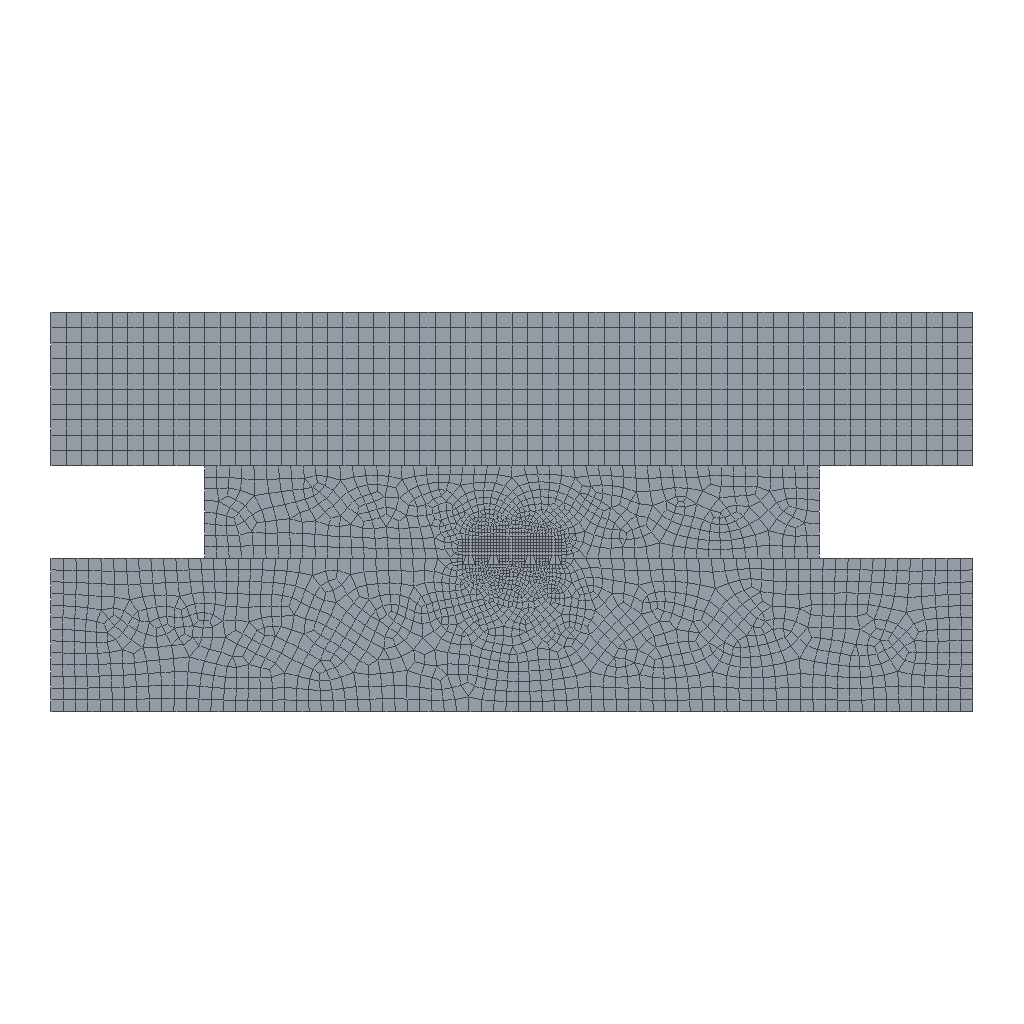Simulation study | abaqus
Set-up summary:
category,name,step,type,value,unit,region
solver,abaqus
solver,version,,,Abaqus/Standard 2020
units,not stated in the deck,,not stated
analysis,deck,,static,static
load_step,Step-1,Step-1,static,nlgeom=True
load_step,Step-2,Step-2,static,nlgeom=True
load_step,Step-3,Step-3,static,nlgeom=True
contact,interactions,,,general=0 pairs=2 ties=0
load_step,requested,,,3
mesh,nodes,,,3315
mesh,elements,,,3098
element_type,CPE3,,plane,75
element_type,CPE4R,,plane,3023
load,load commands in deck,,count,4
bc,support commands in deck,,count,5
material,GLASS,,in results
material,WC,,in results
check,setup vs results,,match,"per instance, exact: element labels, types and connectivity; labels of the nodes the elements use; coordinates of those nodes at SINGLE_PRECISION in 2 of 3 instance(s)"
Abaqus input file, long lists of numbers shortened, first 511 of 1902 lines:
*Heading
** Job name: Job-1 Model name: Model-1
** Generated by: Abaqus/CAE 2020
*Preprint, echo=NO, model=NO, history=NO, contact=NO
**
** PARTS
**
*Part, name="Lower mold"
*Node
      1,   1.629,        -2.75
      2,   1.589,        -2.75
** (1613 more lines like these left out)
*Element, type=CPE3
 1, 1555, 1350, 1575
 2, 1293, 1359, 1182
** (47 more lines like these left out)
*Element, type=CPE4R
  50, 1432,  391,   16,  270
  51,  417,  444,  494, 1443
** (1479 more lines like these left out)
*Node
   1616,         1.75,          -3.,           0.
*Nset, nset="Lower mold-RefPt_", internal
1616,
*Nset, nset=Set-1, generate
    1,  1615,     1
*Elset, elset=Set-1, generate
    1,  1530,     1
** Section: Lower mold
*Solid Section, elset=Set-1, material=WC
,
*End Part
**
*Part, name="Upper mold"
*Node
      1,          3.5,        -2.25
      2,    3.475,        -2.25
** (669 more lines like these left out)
*Element, type=CPE4R
  1,   1,   2,  63,  62
  2,   2,   3,  64,  63
** (598 more lines like these left out)
*Node
    672,         2.75,        -2.25,           0.
*Nset, nset="Upper mold-RefPt_", internal
672,
*Nset, nset=Set-1, generate
   1,  671,    1
*Elset, elset=Set-1, generate
   1,  600,    1
** Section: Upper mold
*Solid Section, elset=Set-1, material=WC
,
*End Part
**
*Part, name=glass
*Node
      1,   2.58,          -3.
      2,   2.58,  -2.97
** (1025 more lines like these left out)
*Element, type=CPE4R
  1,   1,   9, 186,  80
  2,   9,  10, 187, 186
** (940 more lines like these left out)
*Element, type=CPE3
193,  718,  682,  701
194,  377,  961,  378
** (24 more lines like these left out)
*Nset, nset=Set-1, generate
    1,  1027,     1
*Elset, elset=Set-1, generate
   1,  968,    1
** Section: Glass
*Solid Section, elset=Set-1, material=GLASS
,
*End Part
**
**
** ASSEMBLY
**
*Assembly, name=Assembly
**
*Instance, name="Upper mold-1", part="Upper mold"
*End Instance
**
*Instance, name=glass-1, part=glass
        0.25,         0.35,           0.
*End Instance
**
*Instance, name="Lower mold-1", part="Lower mold"
          1.,          0.1,           0.
*End Instance
**
*Nset, nset=Set-6, instance="Lower mold-1"
 1616,
*Nset, nset=Set-7, instance="Upper mold-1"
 672,
*Nset, nset=Set-8, instance="Upper mold-1"
 672,
*Nset, nset=Set-9, instance="Lower mold-1"
 1616,
*Nset, nset=Set-10, instance="Lower mold-1"
 1616,
*Nset, nset=Set-11, instance="Upper mold-1"
 672,
*Nset, nset=Set-12, instance="Upper mold-1"
 672,
*Nset, nset=Set-13, instance="Lower mold-1"
 1616,
*Nset, nset=Set-14, instance="Lower mold-1"
 1616,
*Nset, nset=Set-15, instance="Upper mold-1"
 672,
*Nset, nset=Set-16, instance="Upper mold-1"
 672,
*Nset, nset=Set-17, instance="Lower mold-1"
 1616,
*Nset, nset=Set-18, instance="Lower mold-1"
 1616,
*Nset, nset=Set-19, instance="Upper mold-1"
 672,
*Nset, nset=Set-20, instance="Upper mold-1"
 672,
*Nset, nset=Set-21, instance="Lower mold-1"
 1616,
*Nset, nset=Set-22, instance="Lower mold-1"
 1616,
*Nset, nset=Set-23, instance="Upper mold-1"
 672,
*Nset, nset=Set-24, instance="Upper mold-1"
 672,
*Nset, nset=Set-25, instance="Lower mold-1"
 1616,
*Nset, nset=Set-26, instance="Lower mold-1"
 1616,
*Nset, nset=Set-27, instance="Upper mold-1"
 672,
*Nset, nset=Set-28, instance="Upper mold-1"
 672,
*Nset, nset=Set-29, instance="Lower mold-1"
 1616,
*Nset, nset=Set-30, instance="Lower mold-1"
 1616,
*Nset, nset=Set-31, instance="Upper mold-1"
 672,
*Nset, nset=Set-32, instance="Upper mold-1"
 672,
*Nset, nset=Set-33, instance="Lower mold-1"
 1616,
*Nset, nset=Set-34, instance="Lower mold-1"
 1616,
*Nset, nset=Set-35, instance="Upper mold-1"
 672,
*Nset, nset=Set-36, instance="Upper mold-1"
 672,
*Nset, nset=Set-37, instance="Lower mold-1"
 1616,
*Nset, nset=Set-38, instance="Lower mold-1"
 1616,
*Nset, nset=Set-39, instance="Upper mold-1"
 672,
*Nset, nset=Set-40, instance="Upper mold-1"
 672,
*Nset, nset=Set-41, instance="Lower mold-1"
 1616,
*Nset, nset=Set-42, instance="Lower mold-1"
 1616,
*Nset, nset=Set-43, instance="Upper mold-1"
 672,
*Nset, nset=Set-44, instance="Upper mold-1"
 672,
*Nset, nset=Set-45, instance="Lower mold-1"
 1616,
*Nset, nset=Set-46, instance="Lower mold-1"
 1616,
*Nset, nset=Set-47, instance="Upper mold-1"
 672,
*Nset, nset=Set-48, instance="Upper mold-1"
 672,
*Nset, nset=Set-49, instance="Lower mold-1"
 1616,
*Nset, nset=Set-50, instance="Lower mold-1"
 1616,
*Nset, nset=Set-51, instance="Upper mold-1"
 672,
*Nset, nset=Set-52, instance="Upper mold-1"
 672,
*Nset, nset=Set-53, instance="Lower mold-1"
 1616,
*Nset, nset=Set-54, instance="Lower mold-1"
 1616,
*Nset, nset=Set-55, instance="Upper mold-1"
 672,
*Nset, nset=Set-56, instance="Upper mold-1"
 672,
*Nset, nset=Set-57, instance="Lower mold-1"
 1616,
*Nset, nset=Set-58, instance="Lower mold-1"
 1616,
*Nset, nset=Set-59, instance="Upper mold-1"
 672,
*Nset, nset=Set-61, instance=glass-1, generate
    1,  1027,     1
*Elset, elset=Set-61, instance=glass-1, generate
   1,  968,    1
*Nset, nset=Set-62, instance=glass-1, generate
    1,  1027,     1
*Elset, elset=Set-62, instance=glass-1, generate
   1,  968,    1
*Nset, nset=b_Set-1, instance="Upper mold-1", generate
   1,  671,    1
*Elset, elset=b_Set-1, instance="Upper mold-1", generate
   1,  600,    1
*Nset, nset=b_Set-3, instance="Lower mold-1", generate
    1,  1615,     1
*Elset, elset=b_Set-3, instance="Lower mold-1", generate
    1,  1530,     1
*Nset, nset=_PickedSet9, internal, instance="Upper mold-1"
 672,
*Nset, nset=_PickedSet11, internal, instance="Lower mold-1"
 1616,
*Elset, elset=_Surf-227_S1, internal, instance="Upper mold-1", generate
  1,  60,   1
*Surface, type=ELEMENT, name=Surf-227
_Surf-227_S1, S1
*Elset, elset=_Surf-228_S3, internal, instance="Upper mold-1", generate
 541,  600,    1
*Surface, type=ELEMENT, name=Surf-228
_Surf-228_S3, S3
*Elset, elset=_Surf-229_S1, internal, instance="Upper mold-1", generate
  1,  60,   1
*Surface, type=ELEMENT, name=Surf-229
_Surf-229_S1, S1
*Elset, elset=_Surf-230_S1, internal, instance="Upper mold-1", generate
  1,  60,   1
*Surface, type=ELEMENT, name=Surf-230
_Surf-230_S1, S1
*Elset, elset=_Surf-231_S1, internal, instance="Upper mold-1", generate
  1,  60,   1
*Surface, type=ELEMENT, name=Surf-231
_Surf-231_S1, S1
*Elset, elset=_m_Surf-1_S1, internal, instance=glass-1
 226, 227, 247, 289, 291, 296, 297, 298, 301, 305, 308, 481, 835, 864
*Elset, elset=_m_Surf-1_S3, internal, instance=glass-1
 228, 245, 292, 295, 420, 483, 841, 844
*Elset, elset=_m_Surf-1_S4, internal, instance=glass-1
 309, 316, 317, 327, 351, 360, 366, 393, 402, 403, 414, 484
*Elset, elset=_m_Surf-1_S2, internal, instance=glass-1
 333, 355, 367, 379, 383, 394, 409, 485, 486, 487, 488, 489, 490, 491, 492, 944
*Surface, type=ELEMENT, name=m_Surf-1
_m_Surf-1_S1, S1
_m_Surf-1_S3, S3
_m_Surf-1_S4, S4
_m_Surf-1_S2, S2
*Elset, elset=_m_Surf-3_S3, internal, instance="Lower mold-1"
  50, 190, 462
*Elset, elset=_m_Surf-3_S2, internal, instance="Lower mold-1"
   88,   96,  104,  112,  120,  128,  136,  144,  151,  152,  158,  165,  166,  181,  610, 1053
 1054, 1063, 1064, 1065, 1066, 1068, 1070, 1071
*Elset, elset=_m_Surf-3_S1, internal, instance="Lower mold-1"
 135, 143, 173
*Elset, elset=_m_Surf-3_S4, internal, instance="Lower mold-1"
 189, 461, 463, 474
*Surface, type=ELEMENT, name=m_Surf-3
_m_Surf-3_S3, S3
_m_Surf-3_S2, S2
_m_Surf-3_S4, S4
_m_Surf-3_S1, S1
*Elset, elset=_m_Surf-5_S3, internal, instance="Lower mold-1"
   65,   66,  215,  223,  238,  239,  277,  284,  291,  520,  521,  522,  527, 1080, 1082
*Elset, elset=_m_Surf-5_S1, internal, instance="Lower mold-1"
  216,  224,  231,  246,  253,  269,  303,  516,  518,  519,  524,  525,  747, 1058, 1059, 1079
 1081,
*Elset, elset=_m_Surf-5_S4, internal, instance="Lower mold-1"
 311, 530
*Surface, type=ELEMENT, name=m_Surf-5
_m_Surf-5_S3, S3
_m_Surf-5_S1, S1
_m_Surf-5_S4, S4
*Elset, elset=_m_Surf-7_S2, internal, instance="Lower mold-1"
 328,
*Elset, elset=_m_Surf-7_S4, internal, instance="Lower mold-1"
 329, 555
*Elset, elset=_m_Surf-7_S3, internal, instance="Lower mold-1"
 546,
*Surface, type=ELEMENT, name=m_Surf-7
_m_Surf-7_S2, S2
_m_Surf-7_S4, S4
_m_Surf-7_S3, S3
*Elset, elset=_m_Surf-9_S1, internal, instance="Lower mold-1"
 317, 319, 565
*Elset, elset=_m_Surf-9_S4, internal, instance="Lower mold-1"
 318, 553
*Elset, elset=_m_Surf-9_S3, internal, instance="Lower mold-1"
 540, 541
*Elset, elset=_m_Surf-9_S2, internal, instance="Lower mold-1"
 562,
*Surface, type=ELEMENT, name=m_Surf-9
_m_Surf-9_S1, S1
_m_Surf-9_S4, S4
_m_Surf-9_S2, S2
_m_Surf-9_S3, S3
*Elset, elset=_m_Surf-11_S4, internal, instance="Lower mold-1"
 320, 557
*Elset, elset=_m_Surf-11_S2, internal, instance="Lower mold-1"
 532,
*Elset, elset=_m_Surf-11_S3, internal, instance="Lower mold-1"
 534,
*Surface, type=ELEMENT, name=m_Surf-11
_m_Surf-11_S4, S4
_m_Surf-11_S2, S2
_m_Surf-11_S3, S3
*Elset, elset=_m_Surf-13_S3, internal, instance="Lower mold-1"
  50, 190, 462
*Elset, elset=_m_Surf-13_S2, internal, instance="Lower mold-1"
   88,   96,  104,  112,  120,  128,  136,  144,  151,  152,  158,  165,  166,  181,  610, 1053
 1054, 1063, 1064, 1065, 1066, 1068, 1070, 1071
*Elset, elset=_m_Surf-13_S1, internal, instance="Lower mold-1"
 135, 143, 173
*Elset, elset=_m_Surf-13_S4, internal, instance="Lower mold-1"
 189, 461, 463, 474
*Surface, type=ELEMENT, name=m_Surf-13
_m_Surf-13_S3, S3
_m_Surf-13_S2, S2
_m_Surf-13_S4, S4
_m_Surf-13_S1, S1
*Elset, elset=_m_Surf-15_S3, internal, instance="Lower mold-1"
   65,   66,  215,  223,  238,  239,  277,  284,  291,  520,  521,  522,  527, 1080, 1082
*Elset, elset=_m_Surf-15_S1, internal, instance="Lower mold-1"
  216,  224,  231,  246,  253,  269,  303,  516,  518,  519,  524,  525,  747, 1058, 1059, 1079
 1081,
*Elset, elset=_m_Surf-15_S4, internal, instance="Lower mold-1"
 311, 530
*Surface, type=ELEMENT, name=m_Surf-15
_m_Surf-15_S3, S3
_m_Surf-15_S1, S1
_m_Surf-15_S4, S4
*Elset, elset=_m_Surf-17_S2, internal, instance="Lower mold-1"
 328,
*Elset, elset=_m_Surf-17_S4, internal, instance="Lower mold-1"
 329, 555
*Elset, elset=_m_Surf-17_S3, internal, instance="Lower mold-1"
 546,
*Surface, type=ELEMENT, name=m_Surf-17
_m_Surf-17_S2, S2
_m_Surf-17_S4, S4
_m_Surf-17_S3, S3
*Elset, elset=_m_Surf-19_S1, internal, instance="Lower mold-1"
 317, 319, 565
*Elset, elset=_m_Surf-19_S4, internal, instance="Lower mold-1"
 318, 553
*Elset, elset=_m_Surf-19_S3, internal, instance="Lower mold-1"
 540, 541
*Elset, elset=_m_Surf-19_S2, internal, instance="Lower mold-1"
 562,
*Surface, type=ELEMENT, name=m_Surf-19
_m_Surf-19_S1, S1
_m_Surf-19_S4, S4
_m_Surf-19_S2, S2
_m_Surf-19_S3, S3
*Elset, elset=_m_Surf-21_S4, internal, instance="Lower mold-1"
 320, 557
*Elset, elset=_m_Surf-21_S2, internal, instance="Lower mold-1"
 532,
*Elset, elset=_m_Surf-21_S3, internal, instance="Lower mold-1"
 534,
*Surface, type=ELEMENT, name=m_Surf-21
_m_Surf-21_S4, S4
_m_Surf-21_S2, S2
_m_Surf-21_S3, S3
*Elset, elset=_m_Surf-23_S1, internal, instance=glass-1
 226, 227, 247, 289, 291, 296, 297, 298, 301, 305, 308, 481, 835, 864
*Elset, elset=_m_Surf-23_S3, internal, instance=glass-1
 228, 245, 292, 295, 420, 483, 841, 844
*Elset, elset=_m_Surf-23_S4, internal, instance=glass-1
 309, 316, 317, 327, 351, 360, 366, 393, 402, 403, 414, 484
*Elset, elset=_m_Surf-23_S2, internal, instance=glass-1
 333, 355, 367, 379, 383, 394, 409, 485, 486, 487, 488, 489, 490, 491, 492, 944
*Surface, type=ELEMENT, name=m_Surf-23
_m_Surf-23_S1, S1
_m_Surf-23_S3, S3
_m_Surf-23_S4, S4
_m_Surf-23_S2, S2
*Elset, elset=_m_Surf-25_S1, internal, instance=glass-1
 226, 227, 247, 289, 291, 296, 297, 298, 301, 305, 308, 481, 835, 864
*Elset, elset=_m_Surf-25_S3, internal, instance=glass-1
 228, 245, 292, 295, 420, 483, 841, 844
*Elset, elset=_m_Surf-25_S4, internal, instance=glass-1
 309, 316, 317, 327, 351, 360, 366, 393, 402, 403, 414, 484
*Elset, elset=_m_Surf-25_S2, internal, instance=glass-1
 333, 355, 367, 379, 383, 394, 409, 485, 486, 487, 488, 489, 490, 491, 492, 944
*Surface, type=ELEMENT, name=m_Surf-25
_m_Surf-25_S1, S1
_m_Surf-25_S3, S3
_m_Surf-25_S4, S4
_m_Surf-25_S2, S2
*Elset, elset=_m_Surf-27_S3, internal, instance="Lower mold-1"
  50, 190, 462
*Elset, elset=_m_Surf-27_S2, internal, instance="Lower mold-1"
   88,   96,  104,  112,  120,  128,  136,  144,  151,  152,  158,  165,  166,  181,  610, 1053
 1054, 1063, 1064, 1065, 1066, 1068, 1070, 1071
*Elset, elset=_m_Surf-27_S1, internal, instance="Lower mold-1"
 135, 143, 173
*Elset, elset=_m_Surf-27_S4, internal, instance="Lower mold-1"
 189, 461, 463, 474
*Surface, type=ELEMENT, name=m_Surf-27
_m_Surf-27_S3, S3
_m_Surf-27_S2, S2
_m_Surf-27_S4, S4
_m_Surf-27_S1, S1
*Elset, elset=_m_Surf-29_S2, internal, instance="Lower mold-1"
 328,
*Elset, elset=_m_Surf-29_S4, internal, instance="Lower mold-1"
 329, 555
*Elset, elset=_m_Surf-29_S3, internal, instance="Lower mold-1"
 546,
*Surface, type=ELEMENT, name=m_Surf-29
_m_Surf-29_S2, S2
_m_Surf-29_S4, S4
_m_Surf-29_S3, S3
*Elset, elset=_m_Surf-31_S1, internal, instance="Lower mold-1"
 317, 319, 565
*Elset, elset=_m_Surf-31_S4, internal, instance="Lower mold-1"
 318, 553
*Elset, elset=_m_Surf-31_S3, internal, instance="Lower mold-1"
 540, 541
*Elset, elset=_m_Surf-31_S2, internal, instance="Lower mold-1"
 562,
*Surface, type=ELEMENT, name=m_Surf-31
_m_Surf-31_S1, S1
_m_Surf-31_S4, S4
_m_Surf-31_S2, S2
_m_Surf-31_S3, S3
*Elset, elset=_m_Surf-33_S4, internal, instance="Lower mold-1"
 320, 557
*Elset, elset=_m_Surf-33_S2, internal, instance="Lower mold-1"
 532,
*Elset, elset=_m_Surf-33_S3, internal, instance="Lower mold-1"
 534,
*Surface, type=ELEMENT, name=m_Surf-33
_m_Surf-33_S4, S4
_m_Surf-33_S2, S2
_m_Surf-33_S3, S3
*Elset, elset=_m_Surf-35_S1, internal, instance=glass-1
 226, 227, 247, 289, 291, 296, 297, 298, 301, 305, 308, 481, 835, 864
*Elset, elset=_m_Surf-35_S3, internal, instance=glass-1
 228, 245, 292, 295, 420, 483, 841, 844
*Elset, elset=_m_Surf-35_S4, internal, instance=glass-1
 309, 316, 317, 327, 351, 360, 366, 393, 402, 403, 414, 484
*Elset, elset=_m_Surf-35_S2, internal, instance=glass-1
 333, 355, 367, 379, 383, 394, 409, 485, 486, 487, 488, 489, 490, 491, 492, 944
*Surface, type=ELEMENT, name=m_Surf-35
_m_Surf-35_S1, S1
_m_Surf-35_S3, S3
_m_Surf-35_S4, S4
_m_Surf-35_S2, S2
*Elset, elset=_m_Surf-37_S3, internal, instance="Lower mold-1"
  50, 190, 462
*Elset, elset=_m_Surf-37_S2, internal, instance="Lower mold-1"
   88,   96,  104,  112,  120,  128,  136,  144,  151,  152,  158,  165,  166,  181,  610, 1053
 1054, 1063, 1064, 1065, 1066, 1068, 1070, 1071
*Elset, elset=_m_Surf-37_S1, internal, instance="Lower mold-1"
 135, 143, 173
*Elset, elset=_m_Surf-37_S4, internal, instance="Lower mold-1"
 189, 461, 463, 474
*Surface, type=ELEMENT, name=m_Surf-37
_m_Surf-37_S3, S3
_m_Surf-37_S2, S2
_m_Surf-37_S4, S4
_m_Surf-37_S1, S1
*Elset, elset=_m_Surf-39_S3, internal, instance="Lower mold-1"
   65,   66,  215,  223,  238,  239,  277,  284,  291,  520,  521,  522,  527, 1080, 1082
*Elset, elset=_m_Surf-39_S1, internal, instance="Lower mold-1"
  216,  224,  231,  246,  253,  269,  303,  516,  518,  519,  524,  525,  747, 1058, 1059, 1079
 1081,
*Elset, elset=_m_Surf-39_S4, internal, instance="Lower mold-1"
 311, 530
*Surface, type=ELEMENT, name=m_Surf-39
_m_Surf-39_S3, S3
_m_Surf-39_S1, S1
_m_Surf-39_S4, S4
*Elset, elset=_m_Surf-41_S2, internal, instance="Lower mold-1"
 328,
*Elset, elset=_m_Surf-41_S4, internal, instance="Lower mold-1"
 329, 555
*Elset, elset=_m_Surf-41_S3, internal, instance="Lower mold-1"
 546,
*Surface, type=ELEMENT, name=m_Surf-41
_m_Surf-41_S2, S2
_m_Surf-41_S4, S4
_m_Surf-41_S3, S3
*Elset, elset=_m_Surf-43_S1, internal, instance="Lower mold-1"
 317, 319, 565
*Elset, elset=_m_Surf-43_S4, internal, instance="Lower mold-1"
 318, 553
*Elset, elset=_m_Surf-43_S3, internal, instance="Lower mold-1"
 540, 541
*Elset, elset=_m_Surf-43_S2, internal, instance="Lower mold-1"
 562,
*Surface, type=ELEMENT, name=m_Surf-43
_m_Surf-43_S1, S1
_m_Surf-43_S4, S4
_m_Surf-43_S2, S2
_m_Surf-43_S3, S3
*Elset, elset=_m_Surf-45_S4, internal, instance="Lower mold-1"
 320, 557
*Elset, elset=_m_Surf-45_S2, internal, instance="Lower mold-1"
 532,
*Elset, elset=_m_Surf-45_S3, internal, instance="Lower mold-1"
 534,
*Surface, type=ELEMENT, name=m_Surf-45
Last 833 lines:
*Surface, type=ELEMENT, name=m_Surf-163
_m_Surf-163_S4, S4
_m_Surf-163_S2, S2
_m_Surf-163_S3, S3
*Elset, elset=_m_Surf-165_S3, internal, instance="Lower mold-1"
   65,   66,  215,  223,  238,  239,  277,  284,  291,  520,  521,  522,  527, 1080, 1082
*Elset, elset=_m_Surf-165_S1, internal, instance="Lower mold-1"
  216,  224,  231,  246,  253,  269,  303,  516,  518,  519,  524,  525,  747, 1058, 1059, 1079
 1081,
*Elset, elset=_m_Surf-165_S4, internal, instance="Lower mold-1"
 311, 530
*Surface, type=ELEMENT, name=m_Surf-165
_m_Surf-165_S3, S3
_m_Surf-165_S1, S1
_m_Surf-165_S4, S4
*Elset, elset=_m_Surf-167_S3, internal, instance="Upper mold-1", generate
 541,  600,    1
*Surface, type=ELEMENT, name=m_Surf-167
_m_Surf-167_S3, S3
*Elset, elset=_m_Surf-169_S3, internal, instance="Lower mold-1"
  50, 190, 462
*Elset, elset=_m_Surf-169_S2, internal, instance="Lower mold-1"
   88,   96,  104,  112,  120,  128,  136,  144,  151,  152,  158,  165,  166,  181,  610, 1053
 1054, 1063, 1064, 1065, 1066, 1068, 1070, 1071
*Elset, elset=_m_Surf-169_S1, internal, instance="Lower mold-1"
 135, 143, 173
*Elset, elset=_m_Surf-169_S4, internal, instance="Lower mold-1"
 189, 461, 463, 474
*Surface, type=ELEMENT, name=m_Surf-169
_m_Surf-169_S3, S3
_m_Surf-169_S2, S2
_m_Surf-169_S4, S4
_m_Surf-169_S1, S1
*Elset, elset=_m_Surf-171_S2, internal, instance="Lower mold-1"
 328,
*Elset, elset=_m_Surf-171_S4, internal, instance="Lower mold-1"
 329, 555
*Elset, elset=_m_Surf-171_S3, internal, instance="Lower mold-1"
 546,
*Surface, type=ELEMENT, name=m_Surf-171
_m_Surf-171_S2, S2
_m_Surf-171_S4, S4
_m_Surf-171_S3, S3
*Elset, elset=_m_Surf-173_S1, internal, instance="Lower mold-1"
 317, 319, 565
*Elset, elset=_m_Surf-173_S4, internal, instance="Lower mold-1"
 318, 553
*Elset, elset=_m_Surf-173_S3, internal, instance="Lower mold-1"
 540, 541
*Elset, elset=_m_Surf-173_S2, internal, instance="Lower mold-1"
 562,
*Surface, type=ELEMENT, name=m_Surf-173
_m_Surf-173_S1, S1
_m_Surf-173_S4, S4
_m_Surf-173_S2, S2
_m_Surf-173_S3, S3
*Elset, elset=_m_Surf-175_S4, internal, instance="Lower mold-1"
 320, 557
*Elset, elset=_m_Surf-175_S2, internal, instance="Lower mold-1"
 532,
*Elset, elset=_m_Surf-175_S3, internal, instance="Lower mold-1"
 534,
*Surface, type=ELEMENT, name=m_Surf-175
_m_Surf-175_S4, S4
_m_Surf-175_S2, S2
_m_Surf-175_S3, S3
*Elset, elset=_m_Surf-177_S3, internal, instance="Lower mold-1"
   65,   66,  215,  223,  238,  239,  277,  284,  291,  520,  521,  522,  527, 1080, 1082
*Elset, elset=_m_Surf-177_S1, internal, instance="Lower mold-1"
  216,  224,  231,  246,  253,  269,  303,  516,  518,  519,  524,  525,  747, 1058, 1059, 1079
 1081,
*Elset, elset=_m_Surf-177_S4, internal, instance="Lower mold-1"
 311, 530
*Surface, type=ELEMENT, name=m_Surf-177
_m_Surf-177_S3, S3
_m_Surf-177_S1, S1
_m_Surf-177_S4, S4
*Elset, elset=_m_Surf-179_S3, internal, instance="Upper mold-1", generate
 541,  600,    1
*Surface, type=ELEMENT, name=m_Surf-179
_m_Surf-179_S3, S3
*Elset, elset=_m_Surf-181_S3, internal, instance="Lower mold-1"
  50, 190, 462
*Elset, elset=_m_Surf-181_S2, internal, instance="Lower mold-1"
   88,   96,  104,  112,  120,  128,  136,  144,  151,  152,  158,  165,  166,  181,  610, 1053
 1054, 1063, 1064, 1065, 1066, 1068, 1070, 1071
*Elset, elset=_m_Surf-181_S1, internal, instance="Lower mold-1"
 135, 143, 173
*Elset, elset=_m_Surf-181_S4, internal, instance="Lower mold-1"
 189, 461, 463, 474
*Surface, type=ELEMENT, name=m_Surf-181
_m_Surf-181_S3, S3
_m_Surf-181_S2, S2
_m_Surf-181_S4, S4
_m_Surf-181_S1, S1
*Elset, elset=_m_Surf-183_S2, internal, instance="Lower mold-1"
 328,
*Elset, elset=_m_Surf-183_S4, internal, instance="Lower mold-1"
 329, 555
*Elset, elset=_m_Surf-183_S3, internal, instance="Lower mold-1"
 546,
*Surface, type=ELEMENT, name=m_Surf-183
_m_Surf-183_S2, S2
_m_Surf-183_S4, S4
_m_Surf-183_S3, S3
*Elset, elset=_m_Surf-185_S1, internal, instance="Lower mold-1"
 317, 319, 565
*Elset, elset=_m_Surf-185_S4, internal, instance="Lower mold-1"
 318, 553
*Elset, elset=_m_Surf-185_S3, internal, instance="Lower mold-1"
 540, 541
*Elset, elset=_m_Surf-185_S2, internal, instance="Lower mold-1"
 562,
*Surface, type=ELEMENT, name=m_Surf-185
_m_Surf-185_S1, S1
_m_Surf-185_S4, S4
_m_Surf-185_S2, S2
_m_Surf-185_S3, S3
*Elset, elset=_m_Surf-187_S4, internal, instance="Lower mold-1"
 320, 557
*Elset, elset=_m_Surf-187_S2, internal, instance="Lower mold-1"
 532,
*Elset, elset=_m_Surf-187_S3, internal, instance="Lower mold-1"
 534,
*Surface, type=ELEMENT, name=m_Surf-187
_m_Surf-187_S4, S4
_m_Surf-187_S2, S2
_m_Surf-187_S3, S3
*Elset, elset=_m_Surf-189_S3, internal, instance="Lower mold-1"
   65,   66,  215,  223,  238,  239,  277,  284,  291,  520,  521,  522,  527, 1080, 1082
*Elset, elset=_m_Surf-189_S1, internal, instance="Lower mold-1"
  216,  224,  231,  246,  253,  269,  303,  516,  518,  519,  524,  525,  747, 1058, 1059, 1079
 1081,
*Elset, elset=_m_Surf-189_S4, internal, instance="Lower mold-1"
 311, 530
*Surface, type=ELEMENT, name=m_Surf-189
_m_Surf-189_S3, S3
_m_Surf-189_S1, S1
_m_Surf-189_S4, S4
*Elset, elset=_m_Surf-191_S3, internal, instance="Upper mold-1", generate
 541,  600,    1
*Surface, type=ELEMENT, name=m_Surf-191
_m_Surf-191_S3, S3
*Elset, elset=_m_Surf-193_S3, internal, instance="Lower mold-1"
  50, 190, 462
*Elset, elset=_m_Surf-193_S2, internal, instance="Lower mold-1"
   88,   96,  104,  112,  120,  128,  136,  144,  151,  152,  158,  165,  166,  181,  610, 1053
 1054, 1063, 1064, 1065, 1066, 1068, 1070, 1071
*Elset, elset=_m_Surf-193_S1, internal, instance="Lower mold-1"
 135, 143, 173
*Elset, elset=_m_Surf-193_S4, internal, instance="Lower mold-1"
 189, 461, 463, 474
*Surface, type=ELEMENT, name=m_Surf-193
_m_Surf-193_S3, S3
_m_Surf-193_S2, S2
_m_Surf-193_S4, S4
_m_Surf-193_S1, S1
*Elset, elset=_m_Surf-195_S2, internal, instance="Lower mold-1"
 328,
*Elset, elset=_m_Surf-195_S4, internal, instance="Lower mold-1"
 329, 555
*Elset, elset=_m_Surf-195_S3, internal, instance="Lower mold-1"
 546,
*Surface, type=ELEMENT, name=m_Surf-195
_m_Surf-195_S2, S2
_m_Surf-195_S4, S4
_m_Surf-195_S3, S3
*Elset, elset=_m_Surf-197_S1, internal, instance="Lower mold-1"
 317, 319, 565
*Elset, elset=_m_Surf-197_S4, internal, instance="Lower mold-1"
 318, 553
*Elset, elset=_m_Surf-197_S3, internal, instance="Lower mold-1"
 540, 541
*Elset, elset=_m_Surf-197_S2, internal, instance="Lower mold-1"
 562,
*Surface, type=ELEMENT, name=m_Surf-197
_m_Surf-197_S1, S1
_m_Surf-197_S4, S4
_m_Surf-197_S2, S2
_m_Surf-197_S3, S3
*Elset, elset=_m_Surf-199_S4, internal, instance="Lower mold-1"
 320, 557
*Elset, elset=_m_Surf-199_S2, internal, instance="Lower mold-1"
 532,
*Elset, elset=_m_Surf-199_S3, internal, instance="Lower mold-1"
 534,
*Surface, type=ELEMENT, name=m_Surf-199
_m_Surf-199_S4, S4
_m_Surf-199_S2, S2
_m_Surf-199_S3, S3
*Elset, elset=_m_Surf-201_S3, internal, instance="Lower mold-1"
   65,   66,  215,  223,  238,  239,  277,  284,  291,  520,  521,  522,  527, 1080, 1082
*Elset, elset=_m_Surf-201_S1, internal, instance="Lower mold-1"
  216,  224,  231,  246,  253,  269,  303,  516,  518,  519,  524,  525,  747, 1058, 1059, 1079
 1081,
*Elset, elset=_m_Surf-201_S4, internal, instance="Lower mold-1"
 311, 530
*Surface, type=ELEMENT, name=m_Surf-201
_m_Surf-201_S3, S3
_m_Surf-201_S1, S1
_m_Surf-201_S4, S4
*Elset, elset=_m_Surf-203_S3, internal, instance="Upper mold-1", generate
 541,  600,    1
*Surface, type=ELEMENT, name=m_Surf-203
_m_Surf-203_S3, S3
*Elset, elset=_m_Surf-205_S3, internal, instance="Lower mold-1"
  50, 190, 462
*Elset, elset=_m_Surf-205_S2, internal, instance="Lower mold-1"
   88,   96,  104,  112,  120,  128,  136,  144,  151,  152,  158,  165,  166,  181,  610, 1053
 1054, 1063, 1064, 1065, 1066, 1068, 1070, 1071
*Elset, elset=_m_Surf-205_S1, internal, instance="Lower mold-1"
 135, 143, 173
*Elset, elset=_m_Surf-205_S4, internal, instance="Lower mold-1"
 189, 461, 463, 474
*Surface, type=ELEMENT, name=m_Surf-205
_m_Surf-205_S3, S3
_m_Surf-205_S2, S2
_m_Surf-205_S4, S4
_m_Surf-205_S1, S1
*Elset, elset=_m_Surf-207_S2, internal, instance="Lower mold-1"
 328,
*Elset, elset=_m_Surf-207_S4, internal, instance="Lower mold-1"
 329, 555
*Elset, elset=_m_Surf-207_S3, internal, instance="Lower mold-1"
 546,
*Surface, type=ELEMENT, name=m_Surf-207
_m_Surf-207_S2, S2
_m_Surf-207_S4, S4
_m_Surf-207_S3, S3
*Elset, elset=_m_Surf-209_S1, internal, instance="Lower mold-1"
 317, 319, 565
*Elset, elset=_m_Surf-209_S4, internal, instance="Lower mold-1"
 318, 553
*Elset, elset=_m_Surf-209_S3, internal, instance="Lower mold-1"
 540, 541
*Elset, elset=_m_Surf-209_S2, internal, instance="Lower mold-1"
 562,
*Surface, type=ELEMENT, name=m_Surf-209
_m_Surf-209_S1, S1
_m_Surf-209_S4, S4
_m_Surf-209_S2, S2
_m_Surf-209_S3, S3
*Elset, elset=_m_Surf-211_S4, internal, instance="Lower mold-1"
 320, 557
*Elset, elset=_m_Surf-211_S2, internal, instance="Lower mold-1"
 532,
*Elset, elset=_m_Surf-211_S3, internal, instance="Lower mold-1"
 534,
*Surface, type=ELEMENT, name=m_Surf-211
_m_Surf-211_S4, S4
_m_Surf-211_S2, S2
_m_Surf-211_S3, S3
*Elset, elset=_m_Surf-213_S3, internal, instance="Lower mold-1"
   65,   66,  215,  223,  238,  239,  277,  284,  291,  520,  521,  522,  527, 1080, 1082
*Elset, elset=_m_Surf-213_S1, internal, instance="Lower mold-1"
  216,  224,  231,  246,  253,  269,  303,  516,  518,  519,  524,  525,  747, 1058, 1059, 1079
 1081,
*Elset, elset=_m_Surf-213_S4, internal, instance="Lower mold-1"
 311, 530
*Surface, type=ELEMENT, name=m_Surf-213
_m_Surf-213_S3, S3
_m_Surf-213_S1, S1
_m_Surf-213_S4, S4
*Elset, elset=_m_Surf-215_S3, internal, instance="Upper mold-1", generate
 541,  600,    1
*Surface, type=ELEMENT, name=m_Surf-215
_m_Surf-215_S3, S3
*Elset, elset=_m_Surf-217_S3, internal, instance="Lower mold-1"
  50, 190, 462
*Elset, elset=_m_Surf-217_S2, internal, instance="Lower mold-1"
   88,   96,  104,  112,  120,  128,  136,  144,  151,  152,  158,  165,  166,  181,  610, 1053
 1054, 1063, 1064, 1065, 1066, 1068, 1070, 1071
*Elset, elset=_m_Surf-217_S1, internal, instance="Lower mold-1"
 135, 143, 173
*Elset, elset=_m_Surf-217_S4, internal, instance="Lower mold-1"
 189, 461, 463, 474
*Surface, type=ELEMENT, name=m_Surf-217
_m_Surf-217_S3, S3
_m_Surf-217_S2, S2
_m_Surf-217_S4, S4
_m_Surf-217_S1, S1
*Elset, elset=_m_Surf-219_S2, internal, instance="Lower mold-1"
 328,
*Elset, elset=_m_Surf-219_S4, internal, instance="Lower mold-1"
 329, 555
*Elset, elset=_m_Surf-219_S3, internal, instance="Lower mold-1"
 546,
*Surface, type=ELEMENT, name=m_Surf-219
_m_Surf-219_S2, S2
_m_Surf-219_S4, S4
_m_Surf-219_S3, S3
*Elset, elset=_m_Surf-221_S1, internal, instance="Lower mold-1"
 317, 319, 565
*Elset, elset=_m_Surf-221_S4, internal, instance="Lower mold-1"
 318, 553
*Elset, elset=_m_Surf-221_S3, internal, instance="Lower mold-1"
 540, 541
*Elset, elset=_m_Surf-221_S2, internal, instance="Lower mold-1"
 562,
*Surface, type=ELEMENT, name=m_Surf-221
_m_Surf-221_S1, S1
_m_Surf-221_S4, S4
_m_Surf-221_S2, S2
_m_Surf-221_S3, S3
*Elset, elset=_m_Surf-223_S4, internal, instance="Lower mold-1"
 320, 557
*Elset, elset=_m_Surf-223_S2, internal, instance="Lower mold-1"
 532,
*Elset, elset=_m_Surf-223_S3, internal, instance="Lower mold-1"
 534,
*Surface, type=ELEMENT, name=m_Surf-223
_m_Surf-223_S4, S4
_m_Surf-223_S2, S2
_m_Surf-223_S3, S3
*Elset, elset=_m_Surf-225_S3, internal, instance="Lower mold-1"
   65,   66,  215,  223,  238,  239,  277,  284,  291,  520,  521,  522,  527, 1080, 1082
*Elset, elset=_m_Surf-225_S1, internal, instance="Lower mold-1"
  216,  224,  231,  246,  253,  269,  303,  516,  518,  519,  524,  525,  747, 1058, 1059, 1079
 1081,
*Elset, elset=_m_Surf-225_S4, internal, instance="Lower mold-1"
 311, 530
*Surface, type=ELEMENT, name=m_Surf-225
_m_Surf-225_S3, S3
_m_Surf-225_S1, S1
_m_Surf-225_S4, S4
*Elset, elset=_m_Surf-232_S3, internal, instance="Lower mold-1"
   50,   65,   66,  190,  215,  223,  238,  239,  277,  284,  291,  313,  318,  329,  459,  462
  520,  521,  522,  527,  531,  534,  540,  541,  544,  546,  558, 1080, 1082
*Elset, elset=_m_Surf-232_S2, internal, instance="Lower mold-1"
   50,   88,   96,  104,  112,  120,  128,  136,  144,  151,  152,  158,  165,  166,  181,  315
  328,  333,  529,  532,  535,  542,  548,  550,  562,  568,  572,  584,  610, 1053, 1054, 1063
** (1 more lines like these left out)
*Elset, elset=_m_Surf-232_S1, internal, instance="Lower mold-1"
  135,  143,  173,  216,  224,  231,  246,  253,  269,  303,  317,  319,  516,  518,  519,  524
  525,  530,  532,  543,  552,  565,  566,  575,  747, 1058, 1059, 1079, 1081
*Elset, elset=_m_Surf-232_S4, internal, instance="Lower mold-1"
 189, 311, 318, 320, 329, 330, 461, 463, 474, 530, 534, 536, 541, 545, 546, 553
 555, 556, 557, 560
*Surface, type=ELEMENT, name=m_Surf-232
_m_Surf-232_S3, S3
_m_Surf-232_S2, S2
_m_Surf-232_S4, S4
_m_Surf-232_S1, S1
*Elset, elset=_m_Surf-234_S3, internal, instance="Upper mold-1", generate
 541,  600,    1
*Surface, type=ELEMENT, name=m_Surf-234
_m_Surf-234_S3, S3
*Elset, elset=_s_Surf-1_S3, internal, instance="Upper mold-1", generate
 541,  600,    1
*Surface, type=ELEMENT, name=s_Surf-1
_s_Surf-1_S3, S3
*Elset, elset=_s_Surf-23_S3, internal, instance="Upper mold-1", generate
 541,  600,    1
*Surface, type=ELEMENT, name=s_Surf-23
_s_Surf-23_S3, S3
*Elset, elset=_s_Surf-25_S3, internal, instance="Upper mold-1", generate
 541,  600,    1
*Surface, type=ELEMENT, name=s_Surf-25
_s_Surf-25_S3, S3
*Elset, elset=_s_Surf-35_S3, internal, instance="Upper mold-1", generate
 541,  600,    1
*Surface, type=ELEMENT, name=s_Surf-35
_s_Surf-35_S3, S3
*Elset, elset=_s_Surf-47_S3, internal, instance="Upper mold-1", generate
 541,  600,    1
*Surface, type=ELEMENT, name=s_Surf-47
_s_Surf-47_S3, S3
*Elset, elset=_s_Surf-55_S3, internal, instance="Lower mold-1"
  50, 190, 462
*Elset, elset=_s_Surf-55_S2, internal, instance="Lower mold-1"
   88,   96,  104,  112,  120,  128,  136,  144,  151,  152,  158,  165,  166,  181,  610, 1053
 1054, 1063, 1064, 1065, 1066, 1068, 1070, 1071
*Elset, elset=_s_Surf-55_S1, internal, instance="Lower mold-1"
 135, 143, 173
*Elset, elset=_s_Surf-55_S4, internal, instance="Lower mold-1"
 189, 461, 463, 474
*Surface, type=ELEMENT, name=s_Surf-55
_s_Surf-55_S3, S3
_s_Surf-55_S2, S2
_s_Surf-55_S4, S4
_s_Surf-55_S1, S1
*Elset, elset=_s_Surf-57_S3, internal, instance="Lower mold-1"
   65,   66,  215,  223,  238,  239,  277,  284,  291,  520,  521,  522,  527, 1080, 1082
*Elset, elset=_s_Surf-57_S1, internal, instance="Lower mold-1"
  216,  224,  231,  246,  253,  269,  303,  516,  518,  519,  524,  525,  747, 1058, 1059, 1079
 1081,
*Elset, elset=_s_Surf-57_S4, internal, instance="Lower mold-1"
 311, 530
*Surface, type=ELEMENT, name=s_Surf-57
_s_Surf-57_S3, S3
_s_Surf-57_S1, S1
_s_Surf-57_S4, S4
*Elset, elset=_s_Surf-69_S1, internal, instance=glass-1
 226, 227, 247, 289, 291, 296, 297, 298, 301, 305, 308, 481, 835, 864
*Elset, elset=_s_Surf-69_S3, internal, instance=glass-1
 228, 245, 292, 295, 420, 483, 841, 844
*Elset, elset=_s_Surf-69_S4, internal, instance=glass-1
 309, 316, 317, 327, 351, 360, 366, 393, 402, 403, 414, 484
*Elset, elset=_s_Surf-69_S2, internal, instance=glass-1
 333, 355, 367, 379, 383, 394, 409, 485, 486, 487, 488, 489, 490, 491, 492, 944
*Surface, type=ELEMENT, name=s_Surf-69
_s_Surf-69_S1, S1
_s_Surf-69_S3, S3
_s_Surf-69_S4, S4
_s_Surf-69_S2, S2
*Elset, elset=_s_Surf-71_S1, internal, instance=glass-1
 226, 227, 247, 289, 291, 296, 297, 298, 301, 305, 308, 481, 835, 864
*Elset, elset=_s_Surf-71_S3, internal, instance=glass-1
 228, 245, 292, 295, 420, 483, 841, 844
*Elset, elset=_s_Surf-71_S4, internal, instance=glass-1
 309, 316, 317, 327, 351, 360, 366, 393, 402, 403, 414, 484
*Elset, elset=_s_Surf-71_S2, internal, instance=glass-1
 333, 355, 367, 379, 383, 394, 409, 485, 486, 487, 488, 489, 490, 491, 492, 944
*Surface, type=ELEMENT, name=s_Surf-71
_s_Surf-71_S1, S1
_s_Surf-71_S3, S3
_s_Surf-71_S4, S4
_s_Surf-71_S2, S2
*Elset, elset=_s_Surf-77_S2, internal, instance="Lower mold-1"
 328,
*Elset, elset=_s_Surf-77_S4, internal, instance="Lower mold-1"
 329, 555
*Elset, elset=_s_Surf-77_S3, internal, instance="Lower mold-1"
 546,
*Surface, type=ELEMENT, name=s_Surf-77
_s_Surf-77_S2, S2
_s_Surf-77_S4, S4
_s_Surf-77_S3, S3
*Elset, elset=_s_Surf-79_S1, internal, instance="Lower mold-1"
 317, 319, 565
*Elset, elset=_s_Surf-79_S4, internal, instance="Lower mold-1"
 318, 553
*Elset, elset=_s_Surf-79_S3, internal, instance="Lower mold-1"
 540, 541
*Elset, elset=_s_Surf-79_S2, internal, instance="Lower mold-1"
 562,
*Surface, type=ELEMENT, name=s_Surf-79
_s_Surf-79_S1, S1
_s_Surf-79_S4, S4
_s_Surf-79_S2, S2
_s_Surf-79_S3, S3
*Elset, elset=_s_Surf-81_S4, internal, instance="Lower mold-1"
 320, 557
*Elset, elset=_s_Surf-81_S2, internal, instance="Lower mold-1"
 532,
*Elset, elset=_s_Surf-81_S3, internal, instance="Lower mold-1"
 534,
*Surface, type=ELEMENT, name=s_Surf-81
_s_Surf-81_S4, S4
_s_Surf-81_S2, S2
_s_Surf-81_S3, S3
*Elset, elset=_s_Surf-93_S3, internal, instance="Upper mold-1", generate
 541,  600,    1
*Surface, type=ELEMENT, name=s_Surf-93
_s_Surf-93_S3, S3
*Elset, elset=_s_Surf-95_S1, internal, instance=glass-1
 226, 227, 247, 289, 291, 296, 297, 298, 301, 305, 308, 481, 835, 864
*Elset, elset=_s_Surf-95_S3, internal, instance=glass-1
 228, 245, 292, 295, 420, 483, 841, 844
*Elset, elset=_s_Surf-95_S4, internal, instance=glass-1
 309, 316, 317, 327, 351, 360, 366, 393, 402, 403, 414, 484
*Elset, elset=_s_Surf-95_S2, internal, instance=glass-1
 333, 355, 367, 379, 383, 394, 409, 485, 486, 487, 488, 489, 490, 491, 492, 944
*Surface, type=ELEMENT, name=s_Surf-95
_s_Surf-95_S1, S1
_s_Surf-95_S3, S3
_s_Surf-95_S4, S4
_s_Surf-95_S2, S2
*Elset, elset=_s_Surf-107_S1, internal, instance=glass-1
 226, 227, 247, 289, 291, 296, 297, 298, 301, 305, 308, 481, 835, 864
*Elset, elset=_s_Surf-107_S3, internal, instance=glass-1
 228, 245, 292, 295, 420, 483, 841, 844
*Elset, elset=_s_Surf-107_S4, internal, instance=glass-1
 309, 316, 317, 327, 351, 360, 366, 393, 402, 403, 414, 484
*Elset, elset=_s_Surf-107_S2, internal, instance=glass-1
 333, 355, 367, 379, 383, 394, 409, 485, 486, 487, 488, 489, 490, 491, 492, 944
*Surface, type=ELEMENT, name=s_Surf-107
_s_Surf-107_S1, S1
_s_Surf-107_S3, S3
_s_Surf-107_S4, S4
_s_Surf-107_S2, S2
*Elset, elset=_s_Surf-119_S1, internal, instance=glass-1
 226, 227, 247, 289, 291, 296, 297, 298, 301, 305, 308, 481, 835, 864
*Elset, elset=_s_Surf-119_S3, internal, instance=glass-1
 228, 245, 292, 295, 420, 483, 841, 844
*Elset, elset=_s_Surf-119_S4, internal, instance=glass-1
 309, 316, 317, 327, 351, 360, 366, 393, 402, 403, 414, 484
*Elset, elset=_s_Surf-119_S2, internal, instance=glass-1
 333, 355, 367, 379, 383, 394, 409, 485, 486, 487, 488, 489, 490, 491, 492, 944
*Surface, type=ELEMENT, name=s_Surf-119
_s_Surf-119_S1, S1
_s_Surf-119_S3, S3
_s_Surf-119_S4, S4
_s_Surf-119_S2, S2
*Elset, elset=_s_Surf-131_S1, internal, instance=glass-1
 226, 227, 247, 289, 291, 296, 297, 298, 301, 305, 308, 481, 835, 864
*Elset, elset=_s_Surf-131_S3, internal, instance=glass-1
 228, 245, 292, 295, 420, 483, 841, 844
*Elset, elset=_s_Surf-131_S4, internal, instance=glass-1
 309, 316, 317, 327, 351, 360, 366, 393, 402, 403, 414, 484
*Elset, elset=_s_Surf-131_S2, internal, instance=glass-1
 333, 355, 367, 379, 383, 394, 409, 485, 486, 487, 488, 489, 490, 491, 492, 944
*Surface, type=ELEMENT, name=s_Surf-131
_s_Surf-131_S1, S1
_s_Surf-131_S3, S3
_s_Surf-131_S4, S4
_s_Surf-131_S2, S2
*Elset, elset=_s_Surf-139_S4, internal, instance="Lower mold-1"
 320, 557
*Elset, elset=_s_Surf-139_S2, internal, instance="Lower mold-1"
 532,
*Elset, elset=_s_Surf-139_S3, internal, instance="Lower mold-1"
 534,
*Surface, type=ELEMENT, name=s_Surf-139
_s_Surf-139_S4, S4
_s_Surf-139_S2, S2
_s_Surf-139_S3, S3
*Elset, elset=_s_Surf-143_S1, internal, instance=glass-1
 226, 227, 247, 289, 291, 296, 297, 298, 301, 305, 308, 481, 835, 864
*Elset, elset=_s_Surf-143_S3, internal, instance=glass-1
 228, 245, 292, 295, 420, 483, 841, 844
*Elset, elset=_s_Surf-143_S4, internal, instance=glass-1
 309, 316, 317, 327, 351, 360, 366, 393, 402, 403, 414, 484
*Elset, elset=_s_Surf-143_S2, internal, instance=glass-1
 333, 355, 367, 379, 383, 394, 409, 485, 486, 487, 488, 489, 490, 491, 492, 944
*Surface, type=ELEMENT, name=s_Surf-143
_s_Surf-143_S1, S1
_s_Surf-143_S3, S3
_s_Surf-143_S4, S4
_s_Surf-143_S2, S2
*Elset, elset=_s_Surf-155_S1, internal, instance=glass-1
 226, 227, 247, 289, 291, 296, 297, 298, 301, 305, 308, 481, 835, 864
*Elset, elset=_s_Surf-155_S3, internal, instance=glass-1
 228, 245, 292, 295, 420, 483, 841, 844
*Elset, elset=_s_Surf-155_S4, internal, instance=glass-1
 309, 316, 317, 327, 351, 360, 366, 393, 402, 403, 414, 484
*Elset, elset=_s_Surf-155_S2, internal, instance=glass-1
 333, 355, 367, 379, 383, 394, 409, 485, 486, 487, 488, 489, 490, 491, 492, 944
*Surface, type=ELEMENT, name=s_Surf-155
_s_Surf-155_S1, S1
_s_Surf-155_S3, S3
_s_Surf-155_S4, S4
_s_Surf-155_S2, S2
*Elset, elset=_s_Surf-167_S1, internal, instance=glass-1
 226, 227, 247, 289, 291, 296, 297, 298, 301, 305, 308, 481, 835, 864
*Elset, elset=_s_Surf-167_S3, internal, instance=glass-1
 228, 245, 292, 295, 420, 483, 841, 844
*Elset, elset=_s_Surf-167_S4, internal, instance=glass-1
 309, 316, 317, 327, 351, 360, 366, 393, 402, 403, 414, 484
*Elset, elset=_s_Surf-167_S2, internal, instance=glass-1
 333, 355, 367, 379, 383, 394, 409, 485, 486, 487, 488, 489, 490, 491, 492, 944
*Surface, type=ELEMENT, name=s_Surf-167
_s_Surf-167_S1, S1
_s_Surf-167_S3, S3
_s_Surf-167_S4, S4
_s_Surf-167_S2, S2
*Elset, elset=_s_Surf-179_S1, internal, instance=glass-1
 226, 227, 247, 289, 291, 296, 297, 298, 301, 305, 308, 481, 835, 864
*Elset, elset=_s_Surf-179_S3, internal, instance=glass-1
 228, 245, 292, 295, 420, 483, 841, 844
*Elset, elset=_s_Surf-179_S4, internal, instance=glass-1
 309, 316, 317, 327, 351, 360, 366, 393, 402, 403, 414, 484
*Elset, elset=_s_Surf-179_S2, internal, instance=glass-1
 333, 355, 367, 379, 383, 394, 409, 485, 486, 487, 488, 489, 490, 491, 492, 944
*Surface, type=ELEMENT, name=s_Surf-179
_s_Surf-179_S1, S1
_s_Surf-179_S3, S3
_s_Surf-179_S4, S4
_s_Surf-179_S2, S2
*Elset, elset=_s_Surf-191_S1, internal, instance=glass-1
 226, 227, 247, 289, 291, 296, 297, 298, 301, 305, 308, 481, 835, 864
*Elset, elset=_s_Surf-191_S3, internal, instance=glass-1
 228, 245, 292, 295, 420, 483, 841, 844
*Elset, elset=_s_Surf-191_S4, internal, instance=glass-1
 309, 316, 317, 327, 351, 360, 366, 393, 402, 403, 414, 484
*Elset, elset=_s_Surf-191_S2, internal, instance=glass-1
 333, 355, 367, 379, 383, 394, 409, 485, 486, 487, 488, 489, 490, 491, 492, 944
*Surface, type=ELEMENT, name=s_Surf-191
_s_Surf-191_S1, S1
_s_Surf-191_S3, S3
_s_Surf-191_S4, S4
_s_Surf-191_S2, S2
*Elset, elset=_s_Surf-203_S1, internal, instance=glass-1
 226, 227, 247, 289, 291, 296, 297, 298, 301, 305, 308, 481, 835, 864
*Elset, elset=_s_Surf-203_S3, internal, instance=glass-1
 228, 245, 292, 295, 420, 483, 841, 844
*Elset, elset=_s_Surf-203_S4, internal, instance=glass-1
 309, 316, 317, 327, 351, 360, 366, 393, 402, 403, 414, 484
*Elset, elset=_s_Surf-203_S2, internal, instance=glass-1
 333, 355, 367, 379, 383, 394, 409, 485, 486, 487, 488, 489, 490, 491, 492, 944
*Surface, type=ELEMENT, name=s_Surf-203
_s_Surf-203_S1, S1
_s_Surf-203_S3, S3
_s_Surf-203_S4, S4
_s_Surf-203_S2, S2
*Elset, elset=_s_Surf-215_S1, internal, instance=glass-1
 226, 227, 247, 289, 291, 296, 297, 298, 301, 305, 308, 481, 835, 864
*Elset, elset=_s_Surf-215_S3, internal, instance=glass-1
 228, 245, 292, 295, 420, 483, 841, 844
*Elset, elset=_s_Surf-215_S4, internal, instance=glass-1
 309, 316, 317, 327, 351, 360, 366, 393, 402, 403, 414, 484
*Elset, elset=_s_Surf-215_S2, internal, instance=glass-1
 333, 355, 367, 379, 383, 394, 409, 485, 486, 487, 488, 489, 490, 491, 492, 944
*Surface, type=ELEMENT, name=s_Surf-215
_s_Surf-215_S1, S1
_s_Surf-215_S3, S3
_s_Surf-215_S4, S4
_s_Surf-215_S2, S2
*Elset, elset=_s_Surf-232_S4, internal, instance=glass-1
   1,   7,  13,  19,  25,  31,  37,  43,  49,  55,  61,  67,  73,  79,  85,  91
  97, 103, 109, 115, 121, 127, 133, 139, 145, 151, 157, 163, 169, 175, 181, 187
** (1 more lines like these left out)
*Elset, elset=_s_Surf-232_S3, internal, instance=glass-1
 220, 338, 340, 343, 421, 424, 426, 431, 474, 539
*Elset, elset=_s_Surf-232_S2, internal, instance=glass-1
 222, 234, 273, 278, 476, 477, 478, 822
*Elset, elset=_s_Surf-232_S1, internal, instance=glass-1
 274, 339, 341, 342, 344, 345, 347, 350, 422, 425, 427, 469, 495, 496, 742, 773
*Surface, type=ELEMENT, name=s_Surf-232
_s_Surf-232_S4, S4
_s_Surf-232_S3, S3
_s_Surf-232_S2, S2
_s_Surf-232_S1, S1
*Elset, elset=_s_Surf-234_S1, internal, instance=glass-1
 226, 227, 247, 289, 291, 296, 297, 298, 301, 305, 308, 481, 835, 864
*Elset, elset=_s_Surf-234_S3, internal, instance=glass-1
 228, 245, 292, 295, 420, 483, 841, 844
*Elset, elset=_s_Surf-234_S4, internal, instance=glass-1
 309, 316, 317, 327, 351, 360, 366, 393, 402, 403, 414, 484
*Elset, elset=_s_Surf-234_S2, internal, instance=glass-1
 333, 355, 367, 379, 383, 394, 409, 485, 486, 487, 488, 489, 490, 491, 492, 944
*Surface, type=ELEMENT, name=s_Surf-234
_s_Surf-234_S1, S1
_s_Surf-234_S3, S3
_s_Surf-234_S4, S4
_s_Surf-234_S2, S2
** Constraint: Constraint-1
*Rigid Body, ref node=_PickedSet9, elset=b_Set-1
** Constraint: Constraint-2
*Rigid Body, ref node=_PickedSet11, elset=b_Set-3
*End Assembly
*Amplitude, name=Amp-1
             0.,              0.,            180.,              1.,            240.,              1.
*Amplitude, name=Amp-2, definition=PERIODIC
1,          60000.,              0.,              1.
             1.,              0.
*Amplitude, name=Amp-3
             0.,              0.,             10.,              1.,             70.,              1.
*Amplitude, name=Amp-4
             0.,              0.,             60.,              1.,            120.,              1.
*Amplitude, name=Amp-5
             0.,              1.,             40.,              1.
*Amplitude, name=Amp-6
             0.,              0.,             30.,              1.,             40.,              1.
*Amplitude, name=Amp-7
             0.,              0.,             40.,              1.
*Amplitude, name=Amp-8
             0.,              0.,           1680.,              1.
*Amplitude, name=Amp-9
             0.,              1.,             50.,              1.
*Amplitude, name=Amp-10
             0.,              1.,            180.,           0.868
*Amplitude, name=Amp-11
             0.,              1.,           1680.,           0.588
*Amplitude, name=Amp-12
             0.,              1.,           1680.,              1.
*Amplitude, name=Amp-13
             0.,              0.,           1680.,              0.
**
** MATERIALS
**
*Material, name=GLASS
*Conductivity
 0.8,
*Density
 1.1e-09,
*Elastic, moduli=INSTANTANEOUS
20370., 0.275,   25.
19140., 0.275,  275.
18930., 0.275,  285.
18770., 0.275,  290.
18570., 0.275,  295.
18330., 0.275,  300.
18060., 0.275,  305.
17480., 0.275,  310.
15664., 0.275,  325.
14595., 0.275,  330.
11467., 0.275,  340.
*Expansion
 1.3e-05,
*Specific Heat
 3.3e+08,
*Viscoelastic, time=PRONY
 1.,       0., 0.008894
*Trs
295., 11.441, 107.178
*Material, name=WC
*Conductivity
 166.2,
*Density
 1.56e-08,
*Elastic
550000., 0.2
*Expansion
 4.6e-06,
*Specific Heat
 7.1e+08,
**
** INTERACTION PROPERTIES
**
*Surface Interaction, name=IntProp-1
1.,
*Friction, slip tolerance=0.005
 0.15,
*Surface Behavior, pressure-overclosure=HARD
**
** BOUNDARY CONDITIONS
**
** Name: BC-1 Type: 对称/反对称/完全固定
*Boundary
Set-58, ENCASTRE
**
** INTERACTIONS
**
** Interaction: Int-2
*Contact Pair, interaction=IntProp-1, type=SURFACE TO SURFACE, adjust=0.1
s_Surf-232, m_Surf-232
** Interaction: Int-3
*Contact Pair, interaction=IntProp-1, type=SURFACE TO SURFACE
s_Surf-234, m_Surf-234
** ----------------------------------------------------------------
**
** STEP: Step-1
**
*Step, name=Step-1, nlgeom=YES, inc=1000
*Static, stabilize=0.0002, allsdtol=0.05, continue=NO
0.1, 40., 0.0004, 4.
**
** PREDEFINED FIELDS
**
** Name: Predefined Field-1   Type: Temperature
*Temperature, amplitude=Amp-7
Set-62, 340.
**
** OUTPUT REQUESTS
**
*Restart, write, number interval=1, time marks=NO
**
** FIELD OUTPUT: F-Output-1
**
*Output, field
*Node Output
CF, NT, RF, RM, RT, U, V
*Element Output, directions=YES
E, LE, MISES, MISESMAX, PE, PEEQ, PEEQMAX, PEEQT, PEMAG, PEQC, S, TEMP, TSHR, VE, VEEQ, YIELDPOT
*Contact Output
CDISP, CSTRESS
*Output, history, frequency=0
*End Step
** ----------------------------------------------------------------
**
** STEP: Step-2
**
*Step, name=Step-2, nlgeom=YES, inc=1000
*Static, stabilize=0.0002, allsdtol=0.05, continue=NO
0.1, 1680., 0.00168, 100.
**
** BOUNDARY CONDITIONS
**
** Name: BC-2 Type: 位移/转角
*Boundary, amplitude=Amp-8
Set-59, 1, 1
Set-59, 2, 2, -0.03
Set-59, 6, 6
**
** PREDEFINED FIELDS
**
** Name: Predefined Field-1   Type: Temperature
*Temperature, amplitude=Amp-12
Set-62, 340.
**
** OUTPUT REQUESTS
**
*Restart, write, number interval=1, time marks=NO
**
** FIELD OUTPUT: F-Output-1
**
*Output, field
*Node Output
CF, NT, RF, RM, RT, U, V
*Element Output, directions=YES
E, LE, MISES, MISESMAX, PE, PEEQ, PEEQMAX, PEEQT, PEMAG, PEQC, S, TEMP, TSHR, VE, VEEQ, YIELDPOT
*Contact Output
CDISP, CSTRESS
*Output, history, frequency=0
*End Step
** ----------------------------------------------------------------
**
** STEP: Step-3
**
*Step, name=Step-3, nlgeom=YES, inc=1000
*Static, stabilize=0.0002, allsdtol=0.05, continue=NO
0.1, 1680., 0.0168, 100.
**
** BOUNDARY CONDITIONS
**
** Name: BC-1 Type: 对称/反对称/完全固定
*Boundary, op=NEW
Set-58, ENCASTRE
** Name: BC-2 Type: 位移/转角
*Boundary, op=NEW
**
** PREDEFINED FIELDS
**
** Name: Predefined Field-1   Type: Temperature
*Temperature, amplitude=Amp-11
Set-62, 340.
**
** OUTPUT REQUESTS
**
*Restart, write, number interval=1, time marks=NO
**
** FIELD OUTPUT: F-Output-1
**
*Output, field
*Node Output
CF, NT, RF, RM, RT, U, V
*Element Output, directions=YES
E, LE, MISES, MISESMAX, PE, PEEQ, PEEQMAX, PEEQT, PEMAG, PEQC, S, TEMP, TSHR, VE, VEEQ, YIELDPOT
*Contact Output
CDISP, CSTRESS
*Output, history, frequency=0
*End Step
Results summary:
result,step,,completed,increments=33 time=40.0/40.0
result,step,,completed,increments=33 time=1680.0/1680.0
result,step,,completed,increments=71 time=1680.0/1680.0
result,analysis,,,static
result,last_loadstep,,,3
result,analysis steps,,count,3
result,primary field,,,U
result,reaction total,,FX,0.06175,model units
result,reaction total,,FY,0.8842,model units
result,reaction total,,FZ,0.0,model units